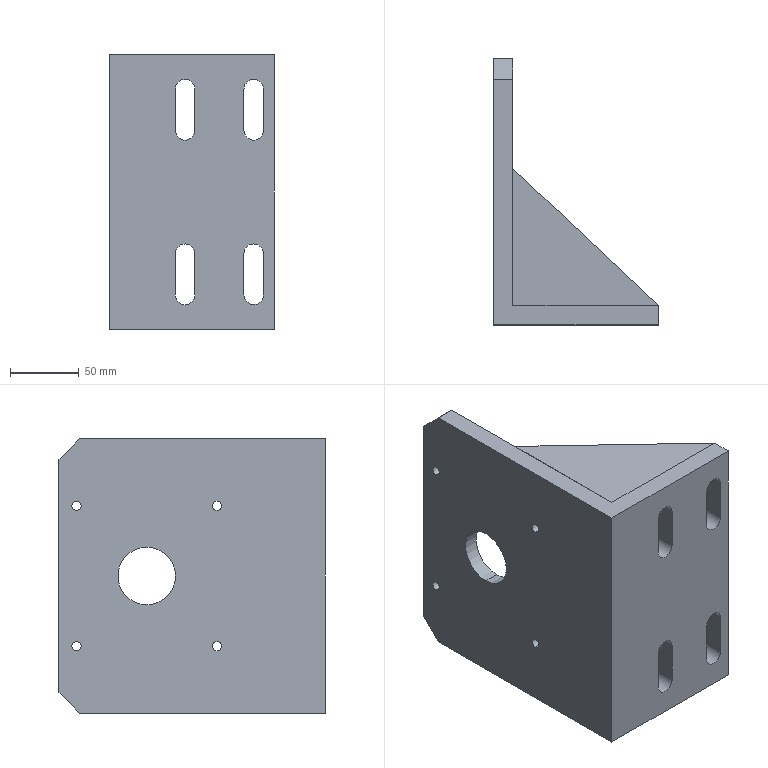Part | SolidWorks | features ICE 7, Chamfer 1, CirPattern 1, Extrusion 1, HoleWzd 1 | 3 solids | 53 faces | box 120 x 194 x 200 mm | volume 863954 mm3 | plane 29 | cylinder 24 | commonest cylinder face diameters 14.332 x12 6.8 x8 42 x2 110 x2